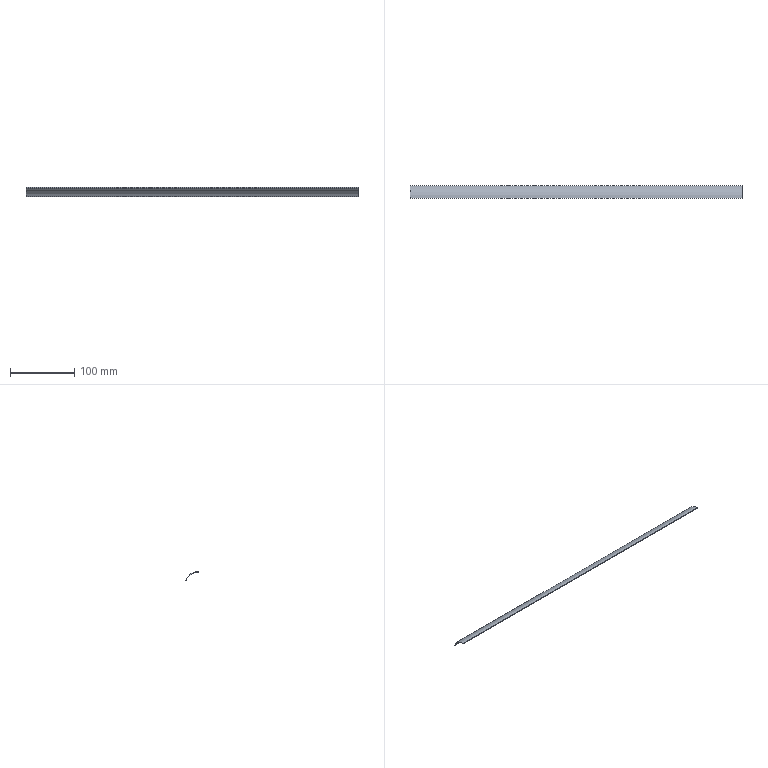Part | STEP file | HESS-408-70-15W-N-18-inner liner louver blade | 1 solid | 6 faces | box 516 x 19.734 x 14.16 mm | volume 12923 mm3 | plane 4 | cylinder 2 | commonest cylinder face diameters 40 x1 42 x1
STEP:
#1=CARTESIAN_POINT('',(0.,0.,0.));
#2=DIRECTION('',(0.,0.,1.));
#3=DIRECTION('',(1.,0.,0.));
#4=AXIS2_PLACEMENT_3D('',#1,#2,#3);
#5=CARTESIAN_POINT('',(258.,0.,21.));
#6=VERTEX_POINT('',#5);
#7=CARTESIAN_POINT('',(258.,19.734,7.182));
#8=VERTEX_POINT('',#7);
#9=CARTESIAN_POINT('',(258.,0.,0.));
#10=DIRECTION('',(-1.,0.,0.));
#11=DIRECTION('',(0.,0.,1.));
#12=AXIS2_PLACEMENT_3D('',#9,#10,#11);
#13=CIRCLE('',#12,21.);
#14=CARTESIAN_POINT('',(258.,0.,0.));
#15=DIRECTION('',(-1.,0.,0.));
#16=DIRECTION('',(0.,0.,1.));
#17=AXIS2_PLACEMENT_3D('',#14,#15,#16);
#18=CYLINDRICAL_SURFACE('',#17,21.);
#19=CARTESIAN_POINT('',(0.,0.));
#20=DIRECTION('',(1.,0.));
#21=VECTOR('',#20,1.);
#22=LINE('',#19,#21);
#23=(GEOMETRIC_REPRESENTATION_CONTEXT(2)PARAMETRIC_REPRESENTATION_CONTEXT()REPRESENTATION_CONTEXT('',''));
#24=DEFINITIONAL_REPRESENTATION('',(#22),#23);
#25=PCURVE('',#18,#24);
#26=CARTESIAN_POINT('',(258.,0.,0.));
#27=DIRECTION('',(1.,0.,0.));
#28=DIRECTION('',(0.,0.,-1.));
#29=AXIS2_PLACEMENT_3D('',#26,#27,#28);
#30=PLANE('',#29);
#31=CARTESIAN_POINT('',(-21.,0.));
#32=CARTESIAN_POINT('',(-21.,36.373));
#33=CARTESIAN_POINT('',(10.5,18.187));
#34=CARTESIAN_POINT('',(42.,0.));
#35=CARTESIAN_POINT('',(10.5,-18.187));
#36=CARTESIAN_POINT('',(-21.,-36.373));
#37=CARTESIAN_POINT('',(-21.,0.));
#38=(BOUNDED_CURVE()B_SPLINE_CURVE(2,(#31,#32,#33,#34,#35,#36,#37),.UNSPECIFIED.,.T.,.F.)B_SPLINE_CURVE_WITH_KNOTS((1,2,2,2,2,1),(-2.094,0.,2.094,4.189,6.283,8.378),.UNSPECIFIED.)CURVE()GEOMETRIC_REPRESENTATION_ITEM()RATIONAL_B_SPLINE_CURVE((1.,0.5,1.,0.5,1.,0.5,1.))REPRESENTATION_ITEM(''));
#39=(GEOMETRIC_REPRESENTATION_CONTEXT(2)PARAMETRIC_REPRESENTATION_CONTEXT()REPRESENTATION_CONTEXT('',''));
#40=DEFINITIONAL_REPRESENTATION('',(#38),#39);
#41=PCURVE('',#30,#40);
#42=SURFACE_CURVE('',#13,(#25,#41),.PCURVE_S1.);
#43=EDGE_CURVE('',#6,#8,#42,.T.);
#44=ORIENTED_EDGE('',*,*,#43,.T.);
#45=CARTESIAN_POINT('',(-258.,19.734,7.182));
#46=VERTEX_POINT('',#45);
#47=CARTESIAN_POINT('',(258.,19.734,7.182));
#48=DIRECTION('',(-1.,0.,0.));
#49=VECTOR('',#48,1.);
#50=LINE('',#47,#49);
#51=CARTESIAN_POINT('',(1.222,0.));
#52=DIRECTION('',(0.,1.));
#53=VECTOR('',#52,1.);
#54=LINE('',#51,#53);
#55=(GEOMETRIC_REPRESENTATION_CONTEXT(2)PARAMETRIC_REPRESENTATION_CONTEXT()REPRESENTATION_CONTEXT('',''));
#56=DEFINITIONAL_REPRESENTATION('',(#54),#55);
#57=PCURVE('',#18,#56);
#58=CARTESIAN_POINT('',(258.,19.734,7.182));
#59=DIRECTION('',(0.,0.342,-0.9397));
#60=DIRECTION('',(0.,0.9397,0.342));
#61=AXIS2_PLACEMENT_3D('',#58,#59,#60);
#62=PLANE('',#61);
#63=CARTESIAN_POINT('',(0.,0.));
#64=DIRECTION('',(0.,-1.));
#65=VECTOR('',#64,1.);
#66=LINE('',#63,#65);
#67=(GEOMETRIC_REPRESENTATION_CONTEXT(2)PARAMETRIC_REPRESENTATION_CONTEXT()REPRESENTATION_CONTEXT('',''));
#68=DEFINITIONAL_REPRESENTATION('',(#66),#67);
#69=PCURVE('',#62,#68);
#70=SURFACE_CURVE('',#50,(#57,#69),.PCURVE_S1.);
#71=EDGE_CURVE('',#8,#46,#70,.T.);
#72=ORIENTED_EDGE('',*,*,#71,.T.);
#73=CARTESIAN_POINT('',(-258.,0.,21.));
#74=VERTEX_POINT('',#73);
#75=CARTESIAN_POINT('',(-258.,0.,0.));
#76=DIRECTION('',(1.,0.,0.));
#77=DIRECTION('',(0.,0.,1.));
#78=AXIS2_PLACEMENT_3D('',#75,#76,#77);
#79=CIRCLE('',#78,21.);
#80=CARTESIAN_POINT('',(6.283,516.));
#81=DIRECTION('',(-1.,0.));
#82=VECTOR('',#81,1.);
#83=LINE('',#80,#82);
#84=(GEOMETRIC_REPRESENTATION_CONTEXT(2)PARAMETRIC_REPRESENTATION_CONTEXT()REPRESENTATION_CONTEXT('',''));
#85=DEFINITIONAL_REPRESENTATION('',(#83),#84);
#86=PCURVE('',#18,#85);
#87=CARTESIAN_POINT('',(-258.,0.,0.));
#88=DIRECTION('',(1.,0.,0.));
#89=DIRECTION('',(0.,0.,-1.));
#90=AXIS2_PLACEMENT_3D('',#87,#88,#89);
#91=PLANE('',#90);
#92=CARTESIAN_POINT('',(0.,0.));
#93=DIRECTION('',(-1.,0.));
#94=AXIS2_PLACEMENT_2D('',#92,#93);
#95=CIRCLE('',#94,21.);
#96=(GEOMETRIC_REPRESENTATION_CONTEXT(2)PARAMETRIC_REPRESENTATION_CONTEXT()REPRESENTATION_CONTEXT('',''));
#97=DEFINITIONAL_REPRESENTATION('',(#95),#96);
#98=PCURVE('',#91,#97);
#99=SURFACE_CURVE('',#79,(#86,#98),.PCURVE_S1.);
#100=EDGE_CURVE('',#46,#74,#99,.T.);
#101=ORIENTED_EDGE('',*,*,#100,.T.);
#102=CARTESIAN_POINT('',(258.,0.,21.));
#103=DIRECTION('',(1.,0.,0.));
#104=VECTOR('',#103,1.);
#105=LINE('',#102,#104);
#106=CARTESIAN_POINT('',(0.,0.));
#107=DIRECTION('',(0.,-1.));
#108=VECTOR('',#107,1.);
#109=LINE('',#106,#108);
#110=(GEOMETRIC_REPRESENTATION_CONTEXT(2)PARAMETRIC_REPRESENTATION_CONTEXT()REPRESENTATION_CONTEXT('',''));
#111=DEFINITIONAL_REPRESENTATION('',(#109),#110);
#112=PCURVE('',#18,#111);
#113=CARTESIAN_POINT('',(258.,0.,20.));
#114=DIRECTION('',(0.,-1.,0.));
#115=DIRECTION('',(0.,0.,-1.));
#116=AXIS2_PLACEMENT_3D('',#113,#114,#115);
#117=PLANE('',#116);
#118=CARTESIAN_POINT('',(-1.,0.));
#119=DIRECTION('',(0.,1.));
#120=VECTOR('',#119,1.);
#121=LINE('',#118,#120);
#122=(GEOMETRIC_REPRESENTATION_CONTEXT(2)PARAMETRIC_REPRESENTATION_CONTEXT()REPRESENTATION_CONTEXT('',''));
#123=DEFINITIONAL_REPRESENTATION('',(#121),#122);
#124=PCURVE('',#117,#123);
#125=SURFACE_CURVE('',#105,(#112,#124),.PCURVE_S1.);
#126=EDGE_CURVE('',#74,#6,#125,.T.);
#127=ORIENTED_EDGE('',*,*,#126,.T.);
#128=EDGE_LOOP('',(#44,#72,#101,#127));
#129=FACE_BOUND('',#128,.T.);
#130=ADVANCED_FACE('',(#129),#18,.T.);
#131=CARTESIAN_POINT('',(258.,18.794,6.84));
#132=VERTEX_POINT('',#131);
#133=CARTESIAN_POINT('',(258.,19.734,7.182));
#134=DIRECTION('',(0.,-0.9397,-0.342));
#135=VECTOR('',#134,1.);
#136=LINE('',#133,#135);
#137=CARTESIAN_POINT('',(0.,0.));
#138=DIRECTION('',(-1.,0.));
#139=VECTOR('',#138,1.);
#140=LINE('',#137,#139);
#141=(GEOMETRIC_REPRESENTATION_CONTEXT(2)PARAMETRIC_REPRESENTATION_CONTEXT()REPRESENTATION_CONTEXT('',''));
#142=DEFINITIONAL_REPRESENTATION('',(#140),#141);
#143=PCURVE('',#62,#142);
#144=CARTESIAN_POINT('',(-7.182,19.734));
#145=DIRECTION('',(0.342,-0.9397));
#146=VECTOR('',#145,1.);
#147=LINE('',#144,#146);
#148=(GEOMETRIC_REPRESENTATION_CONTEXT(2)PARAMETRIC_REPRESENTATION_CONTEXT()REPRESENTATION_CONTEXT('',''));
#149=DEFINITIONAL_REPRESENTATION('',(#147),#148);
#150=PCURVE('',#30,#149);
#151=SURFACE_CURVE('',#136,(#143,#150),.PCURVE_S1.);
#152=EDGE_CURVE('',#8,#132,#151,.T.);
#153=ORIENTED_EDGE('',*,*,#152,.T.);
#154=CARTESIAN_POINT('',(-258.,18.794,6.84));
#155=VERTEX_POINT('',#154);
#156=CARTESIAN_POINT('',(258.,18.794,6.84));
#157=DIRECTION('',(-1.,0.,0.));
#158=VECTOR('',#157,1.);
#159=LINE('',#156,#158);
#160=CARTESIAN_POINT('',(-1.,0.));
#161=DIRECTION('',(0.,-1.));
#162=VECTOR('',#161,1.);
#163=LINE('',#160,#162);
#164=(GEOMETRIC_REPRESENTATION_CONTEXT(2)PARAMETRIC_REPRESENTATION_CONTEXT()REPRESENTATION_CONTEXT('',''));
#165=DEFINITIONAL_REPRESENTATION('',(#163),#164);
#166=PCURVE('',#62,#165);
#167=CARTESIAN_POINT('',(258.,0.,0.));
#168=DIRECTION('',(-1.,0.,0.));
#169=DIRECTION('',(0.,0.,1.));
#170=AXIS2_PLACEMENT_3D('',#167,#168,#169);
#171=CYLINDRICAL_SURFACE('',#170,20.);
#172=CARTESIAN_POINT('',(1.222,0.));
#173=DIRECTION('',(0.,1.));
#174=VECTOR('',#173,1.);
#175=LINE('',#172,#174);
#176=(GEOMETRIC_REPRESENTATION_CONTEXT(2)PARAMETRIC_REPRESENTATION_CONTEXT()REPRESENTATION_CONTEXT('',''));
#177=DEFINITIONAL_REPRESENTATION('',(#175),#176);
#178=PCURVE('',#171,#177);
#179=SURFACE_CURVE('',#159,(#166,#178),.PCURVE_S1.);
#180=EDGE_CURVE('',#132,#155,#179,.T.);
#181=ORIENTED_EDGE('',*,*,#180,.T.);
#182=CARTESIAN_POINT('',(-258.,19.734,7.182));
#183=DIRECTION('',(0.,0.9397,0.342));
#184=VECTOR('',#183,1.);
#185=LINE('',#182,#184);
#186=CARTESIAN_POINT('',(0.,-516.));
#187=DIRECTION('',(1.,0.));
#188=VECTOR('',#187,1.);
#189=LINE('',#186,#188);
#190=(GEOMETRIC_REPRESENTATION_CONTEXT(2)PARAMETRIC_REPRESENTATION_CONTEXT()REPRESENTATION_CONTEXT('',''));
#191=DEFINITIONAL_REPRESENTATION('',(#189),#190);
#192=PCURVE('',#62,#191);
#193=CARTESIAN_POINT('',(-7.182,19.734));
#194=DIRECTION('',(-0.342,0.9397));
#195=VECTOR('',#194,1.);
#196=LINE('',#193,#195);
#197=(GEOMETRIC_REPRESENTATION_CONTEXT(2)PARAMETRIC_REPRESENTATION_CONTEXT()REPRESENTATION_CONTEXT('',''));
#198=DEFINITIONAL_REPRESENTATION('',(#196),#197);
#199=PCURVE('',#91,#198);
#200=SURFACE_CURVE('',#185,(#192,#199),.PCURVE_S1.);
#201=EDGE_CURVE('',#155,#46,#200,.T.);
#202=ORIENTED_EDGE('',*,*,#201,.T.);
#203=ORIENTED_EDGE('',*,*,#71,.F.);
#204=EDGE_LOOP('',(#153,#181,#202,#203));
#205=FACE_BOUND('',#204,.T.);
#206=ADVANCED_FACE('',(#205),#62,.T.);
#207=CARTESIAN_POINT('',(258.,0.,20.));
#208=VERTEX_POINT('',#207);
#209=CARTESIAN_POINT('',(258.,0.,0.));
#210=DIRECTION('',(-1.,0.,0.));
#211=DIRECTION('',(0.,0.,1.));
#212=AXIS2_PLACEMENT_3D('',#209,#210,#211);
#213=CIRCLE('',#212,20.);
#214=CARTESIAN_POINT('',(-20.,0.));
#215=CARTESIAN_POINT('',(-20.,34.641));
#216=CARTESIAN_POINT('',(10.,17.321));
#217=CARTESIAN_POINT('',(40.,0.));
#218=CARTESIAN_POINT('',(10.,-17.321));
#219=CARTESIAN_POINT('',(-20.,-34.641));
#220=CARTESIAN_POINT('',(-20.,0.));
#221=(BOUNDED_CURVE()B_SPLINE_CURVE(2,(#214,#215,#216,#217,#218,#219,#220),.UNSPECIFIED.,.T.,.F.)B_SPLINE_CURVE_WITH_KNOTS((1,2,2,2,2,1),(-2.094,0.,2.094,4.189,6.283,8.378),.UNSPECIFIED.)CURVE()GEOMETRIC_REPRESENTATION_ITEM()RATIONAL_B_SPLINE_CURVE((1.,0.5,1.,0.5,1.,0.5,1.))REPRESENTATION_ITEM(''));
#222=(GEOMETRIC_REPRESENTATION_CONTEXT(2)PARAMETRIC_REPRESENTATION_CONTEXT()REPRESENTATION_CONTEXT('',''));
#223=DEFINITIONAL_REPRESENTATION('',(#221),#222);
#224=PCURVE('',#30,#223);
#225=CARTESIAN_POINT('',(0.,0.));
#226=DIRECTION('',(1.,0.));
#227=VECTOR('',#226,1.);
#228=LINE('',#225,#227);
#229=(GEOMETRIC_REPRESENTATION_CONTEXT(2)PARAMETRIC_REPRESENTATION_CONTEXT()REPRESENTATION_CONTEXT('',''));
#230=DEFINITIONAL_REPRESENTATION('',(#228),#229);
#231=PCURVE('',#171,#230);
#232=SURFACE_CURVE('',#213,(#224,#231),.PCURVE_S1.);
#233=EDGE_CURVE('',#208,#132,#232,.T.);
#234=ORIENTED_EDGE('',*,*,#233,.T.);
#235=ORIENTED_EDGE('',*,*,#152,.F.);
#236=ORIENTED_EDGE('',*,*,#43,.F.);
#237=CARTESIAN_POINT('',(258.,0.,0.));
#238=DIRECTION('',(0.,0.,-1.));
#239=VECTOR('',#238,1.);
#240=LINE('',#237,#239);
#241=CARTESIAN_POINT('',(0.,0.));
#242=DIRECTION('',(1.,0.));
#243=VECTOR('',#242,1.);
#244=LINE('',#241,#243);
#245=(GEOMETRIC_REPRESENTATION_CONTEXT(2)PARAMETRIC_REPRESENTATION_CONTEXT()REPRESENTATION_CONTEXT('',''));
#246=DEFINITIONAL_REPRESENTATION('',(#244),#245);
#247=PCURVE('',#30,#246);
#248=CARTESIAN_POINT('',(20.,0.));
#249=DIRECTION('',(1.,0.));
#250=VECTOR('',#249,1.);
#251=LINE('',#248,#250);
#252=(GEOMETRIC_REPRESENTATION_CONTEXT(2)PARAMETRIC_REPRESENTATION_CONTEXT()REPRESENTATION_CONTEXT('',''));
#253=DEFINITIONAL_REPRESENTATION('',(#251),#252);
#254=PCURVE('',#117,#253);
#255=SURFACE_CURVE('',#240,(#247,#254),.PCURVE_S1.);
#256=EDGE_CURVE('',#6,#208,#255,.T.);
#257=ORIENTED_EDGE('',*,*,#256,.T.);
#258=EDGE_LOOP('',(#234,#235,#236,#257));
#259=FACE_BOUND('',#258,.T.);
#260=ADVANCED_FACE('',(#259),#30,.T.);
#261=ORIENTED_EDGE('',*,*,#256,.F.);
#262=ORIENTED_EDGE('',*,*,#126,.F.);
#263=CARTESIAN_POINT('',(-258.,0.,20.));
#264=VERTEX_POINT('',#263);
#265=CARTESIAN_POINT('',(-258.,0.,20.));
#266=DIRECTION('',(0.,0.,-1.));
#267=VECTOR('',#266,1.);
#268=LINE('',#265,#267);
#269=CARTESIAN_POINT('',(0.,-516.));
#270=DIRECTION('',(1.,0.));
#271=VECTOR('',#270,1.);
#272=LINE('',#269,#271);
#273=(GEOMETRIC_REPRESENTATION_CONTEXT(2)PARAMETRIC_REPRESENTATION_CONTEXT()REPRESENTATION_CONTEXT('',''));
#274=DEFINITIONAL_REPRESENTATION('',(#272),#273);
#275=PCURVE('',#117,#274);
#276=CARTESIAN_POINT('',(-20.,0.));
#277=DIRECTION('',(1.,0.));
#278=VECTOR('',#277,1.);
#279=LINE('',#276,#278);
#280=(GEOMETRIC_REPRESENTATION_CONTEXT(2)PARAMETRIC_REPRESENTATION_CONTEXT()REPRESENTATION_CONTEXT('',''));
#281=DEFINITIONAL_REPRESENTATION('',(#279),#280);
#282=PCURVE('',#91,#281);
#283=SURFACE_CURVE('',#268,(#275,#282),.PCURVE_S1.);
#284=EDGE_CURVE('',#74,#264,#283,.T.);
#285=ORIENTED_EDGE('',*,*,#284,.T.);
#286=CARTESIAN_POINT('',(258.,0.,20.));
#287=DIRECTION('',(1.,0.,0.));
#288=VECTOR('',#287,1.);
#289=LINE('',#286,#288);
#290=CARTESIAN_POINT('',(0.,0.));
#291=DIRECTION('',(0.,1.));
#292=VECTOR('',#291,1.);
#293=LINE('',#290,#292);
#294=(GEOMETRIC_REPRESENTATION_CONTEXT(2)PARAMETRIC_REPRESENTATION_CONTEXT()REPRESENTATION_CONTEXT('',''));
#295=DEFINITIONAL_REPRESENTATION('',(#293),#294);
#296=PCURVE('',#117,#295);
#297=CARTESIAN_POINT('',(0.,0.));
#298=DIRECTION('',(0.,-1.));
#299=VECTOR('',#298,1.);
#300=LINE('',#297,#299);
#301=(GEOMETRIC_REPRESENTATION_CONTEXT(2)PARAMETRIC_REPRESENTATION_CONTEXT()REPRESENTATION_CONTEXT('',''));
#302=DEFINITIONAL_REPRESENTATION('',(#300),#301);
#303=PCURVE('',#171,#302);
#304=SURFACE_CURVE('',#289,(#296,#303),.PCURVE_S1.);
#305=EDGE_CURVE('',#264,#208,#304,.T.);
#306=ORIENTED_EDGE('',*,*,#305,.T.);
#307=EDGE_LOOP('',(#261,#262,#285,#306));
#308=FACE_BOUND('',#307,.T.);
#309=ADVANCED_FACE('',(#308),#117,.T.);
#310=ORIENTED_EDGE('',*,*,#201,.F.);
#311=CARTESIAN_POINT('',(-258.,0.,0.));
#312=DIRECTION('',(-1.,0.,0.));
#313=DIRECTION('',(0.,0.,1.));
#314=AXIS2_PLACEMENT_3D('',#311,#312,#313);
#315=CIRCLE('',#314,20.);
#316=CARTESIAN_POINT('',(-20.,0.));
#317=CARTESIAN_POINT('',(-20.,34.641));
#318=CARTESIAN_POINT('',(10.,17.321));
#319=CARTESIAN_POINT('',(40.,0.));
#320=CARTESIAN_POINT('',(10.,-17.321));
#321=CARTESIAN_POINT('',(-20.,-34.641));
#322=CARTESIAN_POINT('',(-20.,0.));
#323=(BOUNDED_CURVE()B_SPLINE_CURVE(2,(#316,#317,#318,#319,#320,#321,#322),.UNSPECIFIED.,.T.,.F.)B_SPLINE_CURVE_WITH_KNOTS((1,2,2,2,2,1),(-2.094,0.,2.094,4.189,6.283,8.378),.UNSPECIFIED.)CURVE()GEOMETRIC_REPRESENTATION_ITEM()RATIONAL_B_SPLINE_CURVE((1.,0.5,1.,0.5,1.,0.5,1.))REPRESENTATION_ITEM(''));
#324=(GEOMETRIC_REPRESENTATION_CONTEXT(2)PARAMETRIC_REPRESENTATION_CONTEXT()REPRESENTATION_CONTEXT('',''));
#325=DEFINITIONAL_REPRESENTATION('',(#323),#324);
#326=PCURVE('',#91,#325);
#327=CARTESIAN_POINT('',(0.,516.));
#328=DIRECTION('',(1.,0.));
#329=VECTOR('',#328,1.);
#330=LINE('',#327,#329);
#331=(GEOMETRIC_REPRESENTATION_CONTEXT(2)PARAMETRIC_REPRESENTATION_CONTEXT()REPRESENTATION_CONTEXT('',''));
#332=DEFINITIONAL_REPRESENTATION('',(#330),#331);
#333=PCURVE('',#171,#332);
#334=SURFACE_CURVE('',#315,(#326,#333),.PCURVE_S1.);
#335=EDGE_CURVE('',#264,#155,#334,.T.);
#336=ORIENTED_EDGE('',*,*,#335,.F.);
#337=ORIENTED_EDGE('',*,*,#284,.F.);
#338=ORIENTED_EDGE('',*,*,#100,.F.);
#339=EDGE_LOOP('',(#310,#336,#337,#338));
#340=FACE_BOUND('',#339,.T.);
#341=ADVANCED_FACE('',(#340),#91,.F.);
#342=ORIENTED_EDGE('',*,*,#335,.F.);
#343=ORIENTED_EDGE('',*,*,#305,.T.);
#344=ORIENTED_EDGE('',*,*,#233,.T.);
#345=ORIENTED_EDGE('',*,*,#180,.T.);
#346=EDGE_LOOP('',(#342,#343,#344,#345));
#347=FACE_BOUND('',#346,.F.);
#348=ADVANCED_FACE('',(#347),#171,.F.);
#349=CLOSED_SHELL('',(#130,#206,#260,#309,#341,#348));
#350=MANIFOLD_SOLID_BREP('',#349);
#351=(LENGTH_UNIT()NAMED_UNIT(*)SI_UNIT(.MILLI.,.METRE.));
#352=UNCERTAINTY_MEASURE_WITH_UNIT(LENGTH_MEASURE(0.0000001),#351,'','');
#353=(NAMED_UNIT(*)PLANE_ANGLE_UNIT()SI_UNIT($,.RADIAN.));
#354=(NAMED_UNIT(*)SI_UNIT($,.STERADIAN.)SOLID_ANGLE_UNIT());
#355=(GEOMETRIC_REPRESENTATION_CONTEXT(3)GLOBAL_UNCERTAINTY_ASSIGNED_CONTEXT((#352))GLOBAL_UNIT_ASSIGNED_CONTEXT((#351,#353,#354))REPRESENTATION_CONTEXT('',''));
#356=ADVANCED_BREP_SHAPE_REPRESENTATION('',(#4,#350),#355);